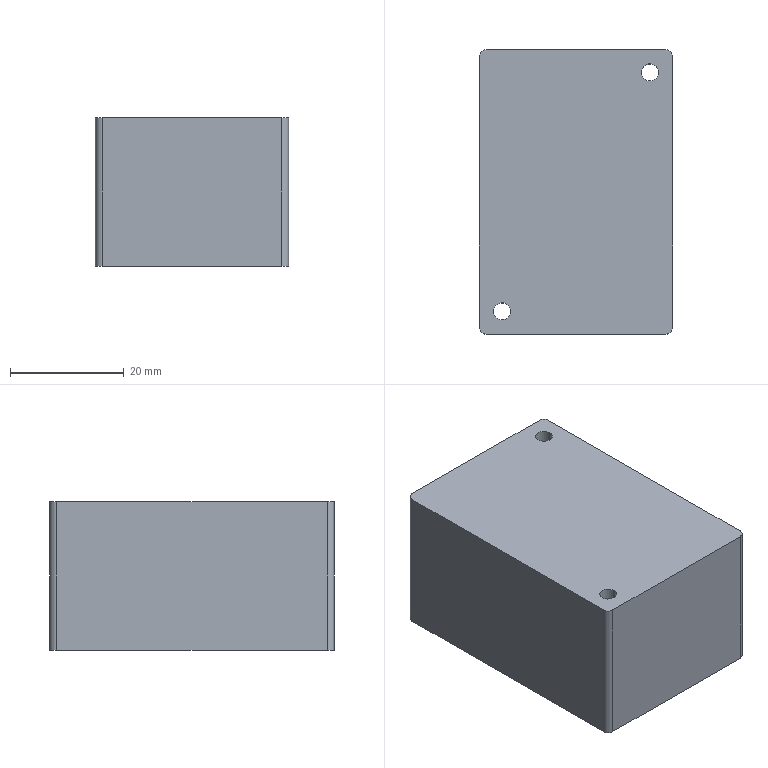Part | STEP file | 4V430C_15_Valve_Switch | 1 solid | 17 faces | box 34 x 50 x 26.2 mm | volume 44112 mm3 | cylinder 10 | plane 7 | commonest cylinder face diameters 2.4 x4 3 x4 3.4 x2
STEP:
#1=CARTESIAN_POINT('',(0.,0.,0.));
#2=DIRECTION('',(0.,0.,1.));
#3=DIRECTION('',(1.,0.,0.));
#4=AXIS2_PLACEMENT_3D('',#1,#2,#3);
#5=CARTESIAN_POINT('',(0.,22.2,-15.9));
#6=VERTEX_POINT('',#5);
#7=CARTESIAN_POINT('',(0.,25.,-15.9));
#8=VERTEX_POINT('',#7);
#9=CARTESIAN_POINT('',(0.,22.2,-15.9));
#10=DIRECTION('',(0.,1.,0.));
#11=VECTOR('',#10,1.);
#12=LINE('',#9,#11);
#13=CARTESIAN_POINT('',(0.,22.2,-17.6));
#14=DIRECTION('',(0.,1.,0.));
#15=DIRECTION('',(0.,0.,1.));
#16=AXIS2_PLACEMENT_3D('',#13,#14,#15);
#17=CYLINDRICAL_SURFACE('',#16,1.7);
#18=CARTESIAN_POINT('',(6.283,0.));
#19=DIRECTION('',(0.,1.));
#20=VECTOR('',#19,1.);
#21=LINE('',#18,#20);
#22=(GEOMETRIC_REPRESENTATION_CONTEXT(2)PARAMETRIC_REPRESENTATION_CONTEXT()REPRESENTATION_CONTEXT('',''));
#23=DEFINITIONAL_REPRESENTATION('',(#21),#22);
#24=PCURVE('',#17,#23);
#25=CARTESIAN_POINT('',(0.,22.2,-17.6));
#26=DIRECTION('',(0.,1.,0.));
#27=DIRECTION('',(0.,0.,1.));
#28=AXIS2_PLACEMENT_3D('',#25,#26,#27);
#29=CYLINDRICAL_SURFACE('',#28,1.7);
#30=CARTESIAN_POINT('',(0.,0.));
#31=DIRECTION('',(0.,1.));
#32=VECTOR('',#31,1.);
#33=LINE('',#30,#32);
#34=(GEOMETRIC_REPRESENTATION_CONTEXT(2)PARAMETRIC_REPRESENTATION_CONTEXT()REPRESENTATION_CONTEXT('',''));
#35=DEFINITIONAL_REPRESENTATION('',(#33),#34);
#36=PCURVE('',#29,#35);
#37=SURFACE_CURVE('',#12,(#24,#36),.PCURVE_S1.);
#38=EDGE_CURVE('',#6,#8,#37,.T.);
#39=ORIENTED_EDGE('',*,*,#38,.T.);
#40=CARTESIAN_POINT('',(0.,25.,-19.3));
#41=VERTEX_POINT('',#40);
#42=CARTESIAN_POINT('',(0.,25.,-17.6));
#43=DIRECTION('',(0.,1.,0.));
#44=DIRECTION('',(0.,0.,1.));
#45=AXIS2_PLACEMENT_3D('',#42,#43,#44);
#46=CIRCLE('',#45,1.7);
#47=CARTESIAN_POINT('',(0.,2.8));
#48=DIRECTION('',(1.,0.));
#49=VECTOR('',#48,1.);
#50=LINE('',#47,#49);
#51=(GEOMETRIC_REPRESENTATION_CONTEXT(2)PARAMETRIC_REPRESENTATION_CONTEXT()REPRESENTATION_CONTEXT('',''));
#52=DEFINITIONAL_REPRESENTATION('',(#50),#51);
#53=PCURVE('',#17,#52);
#54=CARTESIAN_POINT('',(15.8,25.,-26.2));
#55=DIRECTION('',(0.,1.,0.));
#56=DIRECTION('',(0.,0.,1.));
#57=AXIS2_PLACEMENT_3D('',#54,#55,#56);
#58=PLANE('',#57);
#59=CARTESIAN_POINT('',(8.6,-15.8));
#60=DIRECTION('',(1.,0.));
#61=AXIS2_PLACEMENT_2D('',#59,#60);
#62=CIRCLE('',#61,1.7);
#63=(GEOMETRIC_REPRESENTATION_CONTEXT(2)PARAMETRIC_REPRESENTATION_CONTEXT()REPRESENTATION_CONTEXT('',''));
#64=DEFINITIONAL_REPRESENTATION('',(#62),#63);
#65=PCURVE('',#58,#64);
#66=SURFACE_CURVE('',#46,(#53,#65),.PCURVE_S1.);
#67=EDGE_CURVE('',#41,#8,#66,.T.);
#68=ORIENTED_EDGE('',*,*,#67,.F.);
#69=CARTESIAN_POINT('',(0.,22.2,-19.3));
#70=VERTEX_POINT('',#69);
#71=CARTESIAN_POINT('',(0.,22.2,-19.3));
#72=DIRECTION('',(0.,1.,0.));
#73=VECTOR('',#72,1.);
#74=LINE('',#71,#73);
#75=CARTESIAN_POINT('',(3.142,0.));
#76=DIRECTION('',(0.,1.));
#77=VECTOR('',#76,1.);
#78=LINE('',#75,#77);
#79=(GEOMETRIC_REPRESENTATION_CONTEXT(2)PARAMETRIC_REPRESENTATION_CONTEXT()REPRESENTATION_CONTEXT('',''));
#80=DEFINITIONAL_REPRESENTATION('',(#78),#79);
#81=PCURVE('',#17,#80);
#82=CARTESIAN_POINT('',(3.142,0.));
#83=DIRECTION('',(0.,1.));
#84=VECTOR('',#83,1.);
#85=LINE('',#82,#84);
#86=(GEOMETRIC_REPRESENTATION_CONTEXT(2)PARAMETRIC_REPRESENTATION_CONTEXT()REPRESENTATION_CONTEXT('',''));
#87=DEFINITIONAL_REPRESENTATION('',(#85),#86);
#88=PCURVE('',#29,#87);
#89=SURFACE_CURVE('',#74,(#81,#88),.PCURVE_S1.);
#90=EDGE_CURVE('',#70,#41,#89,.T.);
#91=ORIENTED_EDGE('',*,*,#90,.F.);
#92=CARTESIAN_POINT('',(0.,22.2,-17.6));
#93=DIRECTION('',(0.,1.,0.));
#94=DIRECTION('',(0.,0.,1.));
#95=AXIS2_PLACEMENT_3D('',#92,#93,#94);
#96=CIRCLE('',#95,1.7);
#97=CARTESIAN_POINT('',(0.,0.));
#98=DIRECTION('',(1.,0.));
#99=VECTOR('',#98,1.);
#100=LINE('',#97,#99);
#101=(GEOMETRIC_REPRESENTATION_CONTEXT(2)PARAMETRIC_REPRESENTATION_CONTEXT()REPRESENTATION_CONTEXT('',''));
#102=DEFINITIONAL_REPRESENTATION('',(#100),#101);
#103=PCURVE('',#17,#102);
#104=CARTESIAN_POINT('',(0.,22.2,-19.3));
#105=DIRECTION('',(0.,1.,0.));
#106=DIRECTION('',(0.,0.,1.));
#107=AXIS2_PLACEMENT_3D('',#104,#105,#106);
#108=PLANE('',#107);
#109=CARTESIAN_POINT('',(1.7,0.));
#110=DIRECTION('',(1.,0.));
#111=AXIS2_PLACEMENT_2D('',#109,#110);
#112=CIRCLE('',#111,1.7);
#113=(GEOMETRIC_REPRESENTATION_CONTEXT(2)PARAMETRIC_REPRESENTATION_CONTEXT()REPRESENTATION_CONTEXT('',''));
#114=DEFINITIONAL_REPRESENTATION('',(#112),#113);
#115=PCURVE('',#108,#114);
#116=SURFACE_CURVE('',#96,(#103,#115),.PCURVE_S1.);
#117=EDGE_CURVE('',#70,#6,#116,.T.);
#118=ORIENTED_EDGE('',*,*,#117,.T.);
#119=EDGE_LOOP('',(#39,#68,#91,#118));
#120=FACE_BOUND('',#119,.F.);
#121=ADVANCED_FACE('',(#120),#17,.F.);
#122=CARTESIAN_POINT('',(-11.5,-21.,-26.2));
#123=VERTEX_POINT('',#122);
#124=CARTESIAN_POINT('',(-11.5,-21.,0.));
#125=VERTEX_POINT('',#124);
#126=CARTESIAN_POINT('',(-11.5,-21.,-26.2));
#127=DIRECTION('',(0.,0.,1.));
#128=VECTOR('',#127,1.);
#129=LINE('',#126,#128);
#130=CARTESIAN_POINT('',(-13.,-21.,-26.2));
#131=DIRECTION('',(0.,0.,1.));
#132=DIRECTION('',(1.,0.,0.));
#133=AXIS2_PLACEMENT_3D('',#130,#131,#132);
#134=CYLINDRICAL_SURFACE('',#133,1.5);
#135=CARTESIAN_POINT('',(6.283,0.));
#136=DIRECTION('',(0.,1.));
#137=VECTOR('',#136,1.);
#138=LINE('',#135,#137);
#139=(GEOMETRIC_REPRESENTATION_CONTEXT(2)PARAMETRIC_REPRESENTATION_CONTEXT()REPRESENTATION_CONTEXT('',''));
#140=DEFINITIONAL_REPRESENTATION('',(#138),#139);
#141=PCURVE('',#134,#140);
#142=CARTESIAN_POINT('',(-13.,-21.,-26.2));
#143=DIRECTION('',(0.,0.,1.));
#144=DIRECTION('',(1.,0.,0.));
#145=AXIS2_PLACEMENT_3D('',#142,#143,#144);
#146=CYLINDRICAL_SURFACE('',#145,1.5);
#147=CARTESIAN_POINT('',(0.,0.));
#148=DIRECTION('',(0.,1.));
#149=VECTOR('',#148,1.);
#150=LINE('',#147,#149);
#151=(GEOMETRIC_REPRESENTATION_CONTEXT(2)PARAMETRIC_REPRESENTATION_CONTEXT()REPRESENTATION_CONTEXT('',''));
#152=DEFINITIONAL_REPRESENTATION('',(#150),#151);
#153=PCURVE('',#146,#152);
#154=SURFACE_CURVE('',#129,(#141,#153),.PCURVE_S1.);
#155=EDGE_CURVE('',#123,#125,#154,.T.);
#156=ORIENTED_EDGE('',*,*,#155,.T.);
#157=CARTESIAN_POINT('',(-14.5,-21.,0.));
#158=VERTEX_POINT('',#157);
#159=CARTESIAN_POINT('',(-13.,-21.,0.));
#160=DIRECTION('',(0.,0.,1.));
#161=DIRECTION('',(1.,0.,0.));
#162=AXIS2_PLACEMENT_3D('',#159,#160,#161);
#163=CIRCLE('',#162,1.5);
#164=CARTESIAN_POINT('',(0.,26.2));
#165=DIRECTION('',(1.,0.));
#166=VECTOR('',#165,1.);
#167=LINE('',#164,#166);
#168=(GEOMETRIC_REPRESENTATION_CONTEXT(2)PARAMETRIC_REPRESENTATION_CONTEXT()REPRESENTATION_CONTEXT('',''));
#169=DEFINITIONAL_REPRESENTATION('',(#167),#168);
#170=PCURVE('',#134,#169);
#171=CARTESIAN_POINT('',(-15.8,-23.8,0.));
#172=DIRECTION('',(0.,0.,1.));
#173=DIRECTION('',(1.,0.,0.));
#174=AXIS2_PLACEMENT_3D('',#171,#172,#173);
#175=PLANE('',#174);
#176=CARTESIAN_POINT('',(2.8,2.8));
#177=DIRECTION('',(1.,0.));
#178=AXIS2_PLACEMENT_2D('',#176,#177);
#179=CIRCLE('',#178,1.5);
#180=(GEOMETRIC_REPRESENTATION_CONTEXT(2)PARAMETRIC_REPRESENTATION_CONTEXT()REPRESENTATION_CONTEXT('',''));
#181=DEFINITIONAL_REPRESENTATION('',(#179),#180);
#182=PCURVE('',#175,#181);
#183=SURFACE_CURVE('',#163,(#170,#182),.PCURVE_S1.);
#184=EDGE_CURVE('',#158,#125,#183,.T.);
#185=ORIENTED_EDGE('',*,*,#184,.F.);
#186=CARTESIAN_POINT('',(-14.5,-21.,-26.2));
#187=VERTEX_POINT('',#186);
#188=CARTESIAN_POINT('',(-14.5,-21.,-26.2));
#189=DIRECTION('',(0.,0.,1.));
#190=VECTOR('',#189,1.);
#191=LINE('',#188,#190);
#192=CARTESIAN_POINT('',(3.142,0.));
#193=DIRECTION('',(0.,1.));
#194=VECTOR('',#193,1.);
#195=LINE('',#192,#194);
#196=(GEOMETRIC_REPRESENTATION_CONTEXT(2)PARAMETRIC_REPRESENTATION_CONTEXT()REPRESENTATION_CONTEXT('',''));
#197=DEFINITIONAL_REPRESENTATION('',(#195),#196);
#198=PCURVE('',#134,#197);
#199=CARTESIAN_POINT('',(3.142,0.));
#200=DIRECTION('',(0.,1.));
#201=VECTOR('',#200,1.);
#202=LINE('',#199,#201);
#203=(GEOMETRIC_REPRESENTATION_CONTEXT(2)PARAMETRIC_REPRESENTATION_CONTEXT()REPRESENTATION_CONTEXT('',''));
#204=DEFINITIONAL_REPRESENTATION('',(#202),#203);
#205=PCURVE('',#146,#204);
#206=SURFACE_CURVE('',#191,(#198,#205),.PCURVE_S1.);
#207=EDGE_CURVE('',#187,#158,#206,.T.);
#208=ORIENTED_EDGE('',*,*,#207,.F.);
#209=CARTESIAN_POINT('',(-13.,-21.,-26.2));
#210=DIRECTION('',(0.,0.,1.));
#211=DIRECTION('',(1.,0.,0.));
#212=AXIS2_PLACEMENT_3D('',#209,#210,#211);
#213=CIRCLE('',#212,1.5);
#214=CARTESIAN_POINT('',(0.,0.));
#215=DIRECTION('',(1.,0.));
#216=VECTOR('',#215,1.);
#217=LINE('',#214,#216);
#218=(GEOMETRIC_REPRESENTATION_CONTEXT(2)PARAMETRIC_REPRESENTATION_CONTEXT()REPRESENTATION_CONTEXT('',''));
#219=DEFINITIONAL_REPRESENTATION('',(#217),#218);
#220=PCURVE('',#134,#219);
#221=CARTESIAN_POINT('',(-15.8,-23.8,-26.2));
#222=DIRECTION('',(0.,0.,1.));
#223=DIRECTION('',(1.,0.,0.));
#224=AXIS2_PLACEMENT_3D('',#221,#222,#223);
#225=PLANE('',#224);
#226=CARTESIAN_POINT('',(2.8,2.8));
#227=DIRECTION('',(1.,0.));
#228=AXIS2_PLACEMENT_2D('',#226,#227);
#229=CIRCLE('',#228,1.5);
#230=(GEOMETRIC_REPRESENTATION_CONTEXT(2)PARAMETRIC_REPRESENTATION_CONTEXT()REPRESENTATION_CONTEXT('',''));
#231=DEFINITIONAL_REPRESENTATION('',(#229),#230);
#232=PCURVE('',#225,#231);
#233=SURFACE_CURVE('',#213,(#220,#232),.PCURVE_S1.);
#234=EDGE_CURVE('',#187,#123,#233,.T.);
#235=ORIENTED_EDGE('',*,*,#234,.T.);
#236=EDGE_LOOP('',(#156,#185,#208,#235));
#237=FACE_BOUND('',#236,.F.);
#238=ADVANCED_FACE('',(#237),#134,.F.);
#239=CARTESIAN_POINT('',(14.5,21.,-26.2));
#240=VERTEX_POINT('',#239);
#241=CARTESIAN_POINT('',(14.5,21.,0.));
#242=VERTEX_POINT('',#241);
#243=CARTESIAN_POINT('',(14.5,21.,-26.2));
#244=DIRECTION('',(0.,0.,1.));
#245=VECTOR('',#244,1.);
#246=LINE('',#243,#245);
#247=CARTESIAN_POINT('',(13.,21.,-26.2));
#248=DIRECTION('',(0.,0.,1.));
#249=DIRECTION('',(1.,0.,0.));
#250=AXIS2_PLACEMENT_3D('',#247,#248,#249);
#251=CYLINDRICAL_SURFACE('',#250,1.5);
#252=CARTESIAN_POINT('',(6.283,0.));
#253=DIRECTION('',(0.,1.));
#254=VECTOR('',#253,1.);
#255=LINE('',#252,#254);
#256=(GEOMETRIC_REPRESENTATION_CONTEXT(2)PARAMETRIC_REPRESENTATION_CONTEXT()REPRESENTATION_CONTEXT('',''));
#257=DEFINITIONAL_REPRESENTATION('',(#255),#256);
#258=PCURVE('',#251,#257);
#259=CARTESIAN_POINT('',(13.,21.,-26.2));
#260=DIRECTION('',(0.,0.,1.));
#261=DIRECTION('',(1.,0.,0.));
#262=AXIS2_PLACEMENT_3D('',#259,#260,#261);
#263=CYLINDRICAL_SURFACE('',#262,1.5);
#264=CARTESIAN_POINT('',(0.,0.));
#265=DIRECTION('',(0.,1.));
#266=VECTOR('',#265,1.);
#267=LINE('',#264,#266);
#268=(GEOMETRIC_REPRESENTATION_CONTEXT(2)PARAMETRIC_REPRESENTATION_CONTEXT()REPRESENTATION_CONTEXT('',''));
#269=DEFINITIONAL_REPRESENTATION('',(#267),#268);
#270=PCURVE('',#263,#269);
#271=SURFACE_CURVE('',#246,(#258,#270),.PCURVE_S1.);
#272=EDGE_CURVE('',#240,#242,#271,.T.);
#273=ORIENTED_EDGE('',*,*,#272,.T.);
#274=CARTESIAN_POINT('',(11.5,21.,0.));
#275=VERTEX_POINT('',#274);
#276=CARTESIAN_POINT('',(13.,21.,0.));
#277=DIRECTION('',(0.,0.,1.));
#278=DIRECTION('',(1.,0.,0.));
#279=AXIS2_PLACEMENT_3D('',#276,#277,#278);
#280=CIRCLE('',#279,1.5);
#281=CARTESIAN_POINT('',(0.,26.2));
#282=DIRECTION('',(1.,0.));
#283=VECTOR('',#282,1.);
#284=LINE('',#281,#283);
#285=(GEOMETRIC_REPRESENTATION_CONTEXT(2)PARAMETRIC_REPRESENTATION_CONTEXT()REPRESENTATION_CONTEXT('',''));
#286=DEFINITIONAL_REPRESENTATION('',(#284),#285);
#287=PCURVE('',#251,#286);
#288=CARTESIAN_POINT('',(28.8,44.8));
#289=DIRECTION('',(1.,0.));
#290=AXIS2_PLACEMENT_2D('',#288,#289);
#291=CIRCLE('',#290,1.5);
#292=(GEOMETRIC_REPRESENTATION_CONTEXT(2)PARAMETRIC_REPRESENTATION_CONTEXT()REPRESENTATION_CONTEXT('',''));
#293=DEFINITIONAL_REPRESENTATION('',(#291),#292);
#294=PCURVE('',#175,#293);
#295=SURFACE_CURVE('',#280,(#287,#294),.PCURVE_S1.);
#296=EDGE_CURVE('',#275,#242,#295,.T.);
#297=ORIENTED_EDGE('',*,*,#296,.F.);
#298=CARTESIAN_POINT('',(11.5,21.,-26.2));
#299=VERTEX_POINT('',#298);
#300=CARTESIAN_POINT('',(11.5,21.,-26.2));
#301=DIRECTION('',(0.,0.,1.));
#302=VECTOR('',#301,1.);
#303=LINE('',#300,#302);
#304=CARTESIAN_POINT('',(3.142,0.));
#305=DIRECTION('',(0.,1.));
#306=VECTOR('',#305,1.);
#307=LINE('',#304,#306);
#308=(GEOMETRIC_REPRESENTATION_CONTEXT(2)PARAMETRIC_REPRESENTATION_CONTEXT()REPRESENTATION_CONTEXT('',''));
#309=DEFINITIONAL_REPRESENTATION('',(#307),#308);
#310=PCURVE('',#251,#309);
#311=CARTESIAN_POINT('',(3.142,0.));
#312=DIRECTION('',(0.,1.));
#313=VECTOR('',#312,1.);
#314=LINE('',#311,#313);
#315=(GEOMETRIC_REPRESENTATION_CONTEXT(2)PARAMETRIC_REPRESENTATION_CONTEXT()REPRESENTATION_CONTEXT('',''));
#316=DEFINITIONAL_REPRESENTATION('',(#314),#315);
#317=PCURVE('',#263,#316);
#318=SURFACE_CURVE('',#303,(#310,#317),.PCURVE_S1.);
#319=EDGE_CURVE('',#299,#275,#318,.T.);
#320=ORIENTED_EDGE('',*,*,#319,.F.);
#321=CARTESIAN_POINT('',(13.,21.,-26.2));
#322=DIRECTION('',(0.,0.,1.));
#323=DIRECTION('',(1.,0.,0.));
#324=AXIS2_PLACEMENT_3D('',#321,#322,#323);
#325=CIRCLE('',#324,1.5);
#326=CARTESIAN_POINT('',(0.,0.));
#327=DIRECTION('',(1.,0.));
#328=VECTOR('',#327,1.);
#329=LINE('',#326,#328);
#330=(GEOMETRIC_REPRESENTATION_CONTEXT(2)PARAMETRIC_REPRESENTATION_CONTEXT()REPRESENTATION_CONTEXT('',''));
#331=DEFINITIONAL_REPRESENTATION('',(#329),#330);
#332=PCURVE('',#251,#331);
#333=CARTESIAN_POINT('',(28.8,44.8));
#334=DIRECTION('',(1.,0.));
#335=AXIS2_PLACEMENT_2D('',#333,#334);
#336=CIRCLE('',#335,1.5);
#337=(GEOMETRIC_REPRESENTATION_CONTEXT(2)PARAMETRIC_REPRESENTATION_CONTEXT()REPRESENTATION_CONTEXT('',''));
#338=DEFINITIONAL_REPRESENTATION('',(#336),#337);
#339=PCURVE('',#225,#338);
#340=SURFACE_CURVE('',#325,(#332,#339),.PCURVE_S1.);
#341=EDGE_CURVE('',#299,#240,#340,.T.);
#342=ORIENTED_EDGE('',*,*,#341,.T.);
#343=EDGE_LOOP('',(#273,#297,#320,#342));
#344=FACE_BOUND('',#343,.F.);
#345=ADVANCED_FACE('',(#344),#251,.F.);
#346=CARTESIAN_POINT('',(15.8,25.,0.));
#347=VERTEX_POINT('',#346);
#348=CARTESIAN_POINT('',(-15.8,25.,0.));
#349=VERTEX_POINT('',#348);
#350=CARTESIAN_POINT('',(15.8,25.,0.));
#351=DIRECTION('',(-1.,0.,0.));
#352=VECTOR('',#351,1.);
#353=LINE('',#350,#352);
#354=CARTESIAN_POINT('',(26.2,0.));
#355=DIRECTION('',(0.,-1.));
#356=VECTOR('',#355,1.);
#357=LINE('',#354,#356);
#358=(GEOMETRIC_REPRESENTATION_CONTEXT(2)PARAMETRIC_REPRESENTATION_CONTEXT()REPRESENTATION_CONTEXT('',''));
#359=DEFINITIONAL_REPRESENTATION('',(#357),#358);
#360=PCURVE('',#58,#359);
#361=CARTESIAN_POINT('',(31.6,48.8));
#362=DIRECTION('',(-1.,0.));
#363=VECTOR('',#362,1.);
#364=LINE('',#361,#363);
#365=(GEOMETRIC_REPRESENTATION_CONTEXT(2)PARAMETRIC_REPRESENTATION_CONTEXT()REPRESENTATION_CONTEXT('',''));
#366=DEFINITIONAL_REPRESENTATION('',(#364),#365);
#367=PCURVE('',#175,#366);
#368=SURFACE_CURVE('',#353,(#360,#367),.PCURVE_S1.);
#369=EDGE_CURVE('',#347,#349,#368,.T.);
#370=ORIENTED_EDGE('',*,*,#369,.F.);
#371=CARTESIAN_POINT('',(15.8,25.,-26.2));
#372=VERTEX_POINT('',#371);
#373=CARTESIAN_POINT('',(15.8,25.,-26.2));
#374=DIRECTION('',(0.,0.,1.));
#375=VECTOR('',#374,1.);
#376=LINE('',#373,#375);
#377=CARTESIAN_POINT('',(0.,0.));
#378=DIRECTION('',(1.,0.));
#379=VECTOR('',#378,1.);
#380=LINE('',#377,#379);
#381=(GEOMETRIC_REPRESENTATION_CONTEXT(2)PARAMETRIC_REPRESENTATION_CONTEXT()REPRESENTATION_CONTEXT('',''));
#382=DEFINITIONAL_REPRESENTATION('',(#380),#381);
#383=PCURVE('',#58,#382);
#384=CARTESIAN_POINT('',(15.8,23.8,-26.2));
#385=DIRECTION('',(0.,0.,1.));
#386=DIRECTION('',(1.,0.,0.));
#387=AXIS2_PLACEMENT_3D('',#384,#385,#386);
#388=CYLINDRICAL_SURFACE('',#387,1.2);
#389=CARTESIAN_POINT('',(1.571,0.));
#390=DIRECTION('',(0.,1.));
#391=VECTOR('',#390,1.);
#392=LINE('',#389,#391);
#393=(GEOMETRIC_REPRESENTATION_CONTEXT(2)PARAMETRIC_REPRESENTATION_CONTEXT()REPRESENTATION_CONTEXT('',''));
#394=DEFINITIONAL_REPRESENTATION('',(#392),#393);
#395=PCURVE('',#388,#394);
#396=SURFACE_CURVE('',#376,(#383,#395),.PCURVE_S1.);
#397=EDGE_CURVE('',#372,#347,#396,.T.);
#398=ORIENTED_EDGE('',*,*,#397,.F.);
#399=CARTESIAN_POINT('',(-15.8,25.,-26.2));
#400=VERTEX_POINT('',#399);
#401=CARTESIAN_POINT('',(15.8,25.,-26.2));
#402=DIRECTION('',(-1.,0.,0.));
#403=VECTOR('',#402,1.);
#404=LINE('',#401,#403);
#405=CARTESIAN_POINT('',(0.,0.));
#406=DIRECTION('',(0.,-1.));
#407=VECTOR('',#406,1.);
#408=LINE('',#405,#407);
#409=(GEOMETRIC_REPRESENTATION_CONTEXT(2)PARAMETRIC_REPRESENTATION_CONTEXT()REPRESENTATION_CONTEXT('',''));
#410=DEFINITIONAL_REPRESENTATION('',(#408),#409);
#411=PCURVE('',#58,#410);
#412=CARTESIAN_POINT('',(31.6,48.8));
#413=DIRECTION('',(-1.,0.));
#414=VECTOR('',#413,1.);
#415=LINE('',#412,#414);
#416=(GEOMETRIC_REPRESENTATION_CONTEXT(2)PARAMETRIC_REPRESENTATION_CONTEXT()REPRESENTATION_CONTEXT('',''));
#417=DEFINITIONAL_REPRESENTATION('',(#415),#416);
#418=PCURVE('',#225,#417);
#419=SURFACE_CURVE('',#404,(#411,#418),.PCURVE_S1.);
#420=EDGE_CURVE('',#372,#400,#419,.T.);
#421=ORIENTED_EDGE('',*,*,#420,.T.);
#422=CARTESIAN_POINT('',(-15.8,25.,-26.2));
#423=DIRECTION('',(0.,0.,1.));
#424=VECTOR('',#423,1.);
#425=LINE('',#422,#424);
#426=CARTESIAN_POINT('',(0.,-31.6));
#427=DIRECTION('',(1.,0.));
#428=VECTOR('',#427,1.);
#429=LINE('',#426,#428);
#430=(GEOMETRIC_REPRESENTATION_CONTEXT(2)PARAMETRIC_REPRESENTATION_CONTEXT()REPRESENTATION_CONTEXT('',''));
#431=DEFINITIONAL_REPRESENTATION('',(#429),#430);
#432=PCURVE('',#58,#431);
#433=CARTESIAN_POINT('',(-15.8,23.8,-26.2));
#434=DIRECTION('',(0.,0.,1.));
#435=DIRECTION('',(1.,0.,0.));
#436=AXIS2_PLACEMENT_3D('',#433,#434,#435);
#437=CYLINDRICAL_SURFACE('',#436,1.2);
#438=CARTESIAN_POINT('',(1.571,0.));
#439=DIRECTION('',(0.,1.));
#440=VECTOR('',#439,1.);
#441=LINE('',#438,#440);
#442=(GEOMETRIC_REPRESENTATION_CONTEXT(2)PARAMETRIC_REPRESENTATION_CONTEXT()REPRESENTATION_CONTEXT('',''));
#443=DEFINITIONAL_REPRESENTATION('',(#441),#442);
#444=PCURVE('',#437,#443);
#445=SURFACE_CURVE('',#425,(#432,#444),.PCURVE_S1.);
#446=EDGE_CURVE('',#400,#349,#445,.T.);
#447=ORIENTED_EDGE('',*,*,#446,.T.);
#448=EDGE_LOOP('',(#370,#398,#421,#447));
#449=FACE_BOUND('',#448,.T.);
#450=CARTESIAN_POINT('',(0.,25.,-17.6));
#451=DIRECTION('',(0.,1.,0.));
#452=DIRECTION('',(0.,0.,1.));
#453=AXIS2_PLACEMENT_3D('',#450,#451,#452);
#454=CIRCLE('',#453,1.7);
#455=CARTESIAN_POINT('',(8.6,-15.8));
#456=DIRECTION('',(1.,0.));
#457=AXIS2_PLACEMENT_2D('',#455,#456);
#458=CIRCLE('',#457,1.7);
#459=(GEOMETRIC_REPRESENTATION_CONTEXT(2)PARAMETRIC_REPRESENTATION_CONTEXT()REPRESENTATION_CONTEXT('',''));
#460=DEFINITIONAL_REPRESENTATION('',(#458),#459);
#461=PCURVE('',#58,#460);
#462=CARTESIAN_POINT('',(0.,2.8));
#463=DIRECTION('',(1.,0.));
#464=VECTOR('',#463,1.);
#465=LINE('',#462,#464);
#466=(GEOMETRIC_REPRESENTATION_CONTEXT(2)PARAMETRIC_REPRESENTATION_CONTEXT()REPRESENTATION_CONTEXT('',''));
#467=DEFINITIONAL_REPRESENTATION('',(#465),#466);
#468=PCURVE('',#29,#467);
#469=SURFACE_CURVE('',#454,(#461,#468),.PCURVE_S1.);
#470=EDGE_CURVE('',#8,#41,#469,.T.);
#471=ORIENTED_EDGE('',*,*,#470,.F.);
#472=ORIENTED_EDGE('',*,*,#67,.F.);
#473=EDGE_LOOP('',(#471,#472));
#474=FACE_BOUND('',#473,.T.);
#475=ADVANCED_FACE('',(#449,#474),#58,.T.);
#476=CARTESIAN_POINT('',(-17.,-23.8,0.));
#477=VERTEX_POINT('',#476);
#478=CARTESIAN_POINT('',(-15.8,-25.,0.));
#479=VERTEX_POINT('',#478);
#480=CARTESIAN_POINT('',(-15.8,-23.8,0.));
#481=DIRECTION('',(0.,0.,1.));
#482=DIRECTION('',(1.,0.,0.));
#483=AXIS2_PLACEMENT_3D('',#480,#481,#482);
#484=CIRCLE('',#483,1.2);
#485=CARTESIAN_POINT('',(-15.8,-23.8,-26.2));
#486=DIRECTION('',(0.,0.,1.));
#487=DIRECTION('',(1.,0.,0.));
#488=AXIS2_PLACEMENT_3D('',#485,#486,#487);
#489=CYLINDRICAL_SURFACE('',#488,1.2);
#490=CARTESIAN_POINT('',(0.,26.2));
#491=DIRECTION('',(1.,0.));
#492=VECTOR('',#491,1.);
#493=LINE('',#490,#492);
#494=(GEOMETRIC_REPRESENTATION_CONTEXT(2)PARAMETRIC_REPRESENTATION_CONTEXT()REPRESENTATION_CONTEXT('',''));
#495=DEFINITIONAL_REPRESENTATION('',(#493),#494);
#496=PCURVE('',#489,#495);
#497=CARTESIAN_POINT('',(0.,0.));
#498=DIRECTION('',(1.,0.));
#499=AXIS2_PLACEMENT_2D('',#497,#498);
#500=CIRCLE('',#499,1.2);
#501=(GEOMETRIC_REPRESENTATION_CONTEXT(2)PARAMETRIC_REPRESENTATION_CONTEXT()REPRESENTATION_CONTEXT('',''));
#502=DEFINITIONAL_REPRESENTATION('',(#500),#501);
#503=PCURVE('',#175,#502);
#504=SURFACE_CURVE('',#484,(#496,#503),.PCURVE_S1.);
#505=EDGE_CURVE('',#477,#479,#504,.T.);
#506=ORIENTED_EDGE('',*,*,#505,.F.);
#507=CARTESIAN_POINT('',(-17.,-23.8,-26.2));
#508=VERTEX_POINT('',#507);
#509=CARTESIAN_POINT('',(-17.,-23.8,-26.2));
#510=DIRECTION('',(0.,0.,1.));
#511=VECTOR('',#510,1.);
#512=LINE('',#509,#511);
#513=CARTESIAN_POINT('',(3.142,0.));
#514=DIRECTION('',(0.,1.));
#515=VECTOR('',#514,1.);
#516=LINE('',#513,#515);
#517=(GEOMETRIC_REPRESENTATION_CONTEXT(2)PARAMETRIC_REPRESENTATION_CONTEXT()REPRESENTATION_CONTEXT('',''));
#518=DEFINITIONAL_REPRESENTATION('',(#516),#517);
#519=PCURVE('',#489,#518);
#520=CARTESIAN_POINT('',(-17.,23.8,-26.2));
#521=DIRECTION('',(-1.,0.,0.));
#522=DIRECTION('',(0.,0.,1.));
#523=AXIS2_PLACEMENT_3D('',#520,#521,#522);
#524=PLANE('',#523);
#525=CARTESIAN_POINT('',(0.,-47.6));
#526=DIRECTION('',(1.,0.));
#527=VECTOR('',#526,1.);
#528=LINE('',#525,#527);
#529=(GEOMETRIC_REPRESENTATION_CONTEXT(2)PARAMETRIC_REPRESENTATION_CONTEXT()REPRESENTATION_CONTEXT('',''));
#530=DEFINITIONAL_REPRESENTATION('',(#528),#529);
#531=PCURVE('',#524,#530);
#532=SURFACE_CURVE('',#512,(#519,#531),.PCURVE_S1.);
#533=EDGE_CURVE('',#508,#477,#532,.T.);
#534=ORIENTED_EDGE('',*,*,#533,.F.);
#535=CARTESIAN_POINT('',(-15.8,-25.,-26.2));
#536=VERTEX_POINT('',#535);
#537=CARTESIAN_POINT('',(-15.8,-23.8,-26.2));
#538=DIRECTION('',(0.,0.,1.));
#539=DIRECTION('',(1.,0.,0.));
#540=AXIS2_PLACEMENT_3D('',#537,#538,#539);
#541=CIRCLE('',#540,1.2);
#542=CARTESIAN_POINT('',(0.,0.));
#543=DIRECTION('',(1.,0.));
#544=VECTOR('',#543,1.);
#545=LINE('',#542,#544);
#546=(GEOMETRIC_REPRESENTATION_CONTEXT(2)PARAMETRIC_REPRESENTATION_CONTEXT()REPRESENTATION_CONTEXT('',''));
#547=DEFINITIONAL_REPRESENTATION('',(#545),#546);
#548=PCURVE('',#489,#547);
#549=CARTESIAN_POINT('',(0.,0.));
#550=DIRECTION('',(1.,0.));
#551=AXIS2_PLACEMENT_2D('',#549,#550);
#552=CIRCLE('',#551,1.2);
#553=(GEOMETRIC_REPRESENTATION_CONTEXT(2)PARAMETRIC_REPRESENTATION_CONTEXT()REPRESENTATION_CONTEXT('',''));
#554=DEFINITIONAL_REPRESENTATION('',(#552),#553);
#555=PCURVE('',#225,#554);
#556=SURFACE_CURVE('',#541,(#548,#555),.PCURVE_S1.);
#557=EDGE_CURVE('',#508,#536,#556,.T.);
#558=ORIENTED_EDGE('',*,*,#557,.T.);
#559=CARTESIAN_POINT('',(-15.8,-25.,-26.2));
#560=DIRECTION('',(0.,0.,1.));
#561=VECTOR('',#560,1.);
#562=LINE('',#559,#561);
#563=CARTESIAN_POINT('',(4.712,0.));
#564=DIRECTION('',(0.,1.));
#565=VECTOR('',#564,1.);
#566=LINE('',#563,#565);
#567=(GEOMETRIC_REPRESENTATION_CONTEXT(2)PARAMETRIC_REPRESENTATION_CONTEXT()REPRESENTATION_CONTEXT('',''));
#568=DEFINITIONAL_REPRESENTATION('',(#566),#567);
#569=PCURVE('',#489,#568);
#570=CARTESIAN_POINT('',(-15.8,-25.,-26.2));
#571=DIRECTION('',(0.,-1.,0.));
#572=DIRECTION('',(0.,0.,-1.));
#573=AXIS2_PLACEMENT_3D('',#570,#571,#572);
#574=PLANE('',#573);
#575=CARTESIAN_POINT('',(0.,0.));
#576=DIRECTION('',(-1.,0.));
#577=VECTOR('',#576,1.);
#578=LINE('',#575,#577);
#579=(GEOMETRIC_REPRESENTATION_CONTEXT(2)PARAMETRIC_REPRESENTATION_CONTEXT()REPRESENTATION_CONTEXT('',''));
#580=DEFINITIONAL_REPRESENTATION('',(#578),#579);
#581=PCURVE('',#574,#580);
#582=SURFACE_CURVE('',#562,(#569,#581),.PCURVE_S1.);
#583=EDGE_CURVE('',#536,#479,#582,.T.);
#584=ORIENTED_EDGE('',*,*,#583,.T.);
#585=EDGE_LOOP('',(#506,#534,#558,#584));
#586=FACE_BOUND('',#585,.T.);
#587=ADVANCED_FACE('',(#586),#489,.T.);
#588=CARTESIAN_POINT('',(-17.,23.8,0.));
#589=VERTEX_POINT('',#588);
#590=CARTESIAN_POINT('',(-17.,23.8,0.));
#591=DIRECTION('',(0.,-1.,0.));
#592=VECTOR('',#591,1.);
#593=LINE('',#590,#592);
#594=CARTESIAN_POINT('',(26.2,0.));
#595=DIRECTION('',(0.,-1.));
#596=VECTOR('',#595,1.);
#597=LINE('',#594,#596);
#598=(GEOMETRIC_REPRESENTATION_CONTEXT(2)PARAMETRIC_REPRESENTATION_CONTEXT()REPRESENTATION_CONTEXT('',''));
#599=DEFINITIONAL_REPRESENTATION('',(#597),#598);
#600=PCURVE('',#524,#599);
#601=CARTESIAN_POINT('',(-1.2,47.6));
#602=DIRECTION('',(0.,-1.));
#603=VECTOR('',#602,1.);
#604=LINE('',#601,#603);
#605=(GEOMETRIC_REPRESENTATION_CONTEXT(2)PARAMETRIC_REPRESENTATION_CONTEXT()REPRESENTATION_CONTEXT('',''));
#606=DEFINITIONAL_REPRESENTATION('',(#604),#605);
#607=PCURVE('',#175,#606);
#608=SURFACE_CURVE('',#593,(#600,#607),.PCURVE_S1.);
#609=EDGE_CURVE('',#589,#477,#608,.T.);
#610=ORIENTED_EDGE('',*,*,#609,.F.);
#611=CARTESIAN_POINT('',(-17.,23.8,-26.2));
#612=VERTEX_POINT('',#611);
#613=CARTESIAN_POINT('',(-17.,23.8,-26.2));
#614=DIRECTION('',(0.,0.,1.));
#615=VECTOR('',#614,1.);
#616=LINE('',#613,#615);
#617=CARTESIAN_POINT('',(0.,0.));
#618=DIRECTION('',(1.,0.));
#619=VECTOR('',#618,1.);
#620=LINE('',#617,#619);
#621=(GEOMETRIC_REPRESENTATION_CONTEXT(2)PARAMETRIC_REPRESENTATION_CONTEXT()REPRESENTATION_CONTEXT('',''));
#622=DEFINITIONAL_REPRESENTATION('',(#620),#621);
#623=PCURVE('',#524,#622);
#624=CARTESIAN_POINT('',(3.142,0.));
#625=DIRECTION('',(0.,1.));
#626=VECTOR('',#625,1.);
#627=LINE('',#624,#626);
#628=(GEOMETRIC_REPRESENTATION_CONTEXT(2)PARAMETRIC_REPRESENTATION_CONTEXT()REPRESENTATION_CONTEXT('',''));
#629=DEFINITIONAL_REPRESENTATION('',(#627),#628);
#630=PCURVE('',#437,#629);
#631=SURFACE_CURVE('',#616,(#623,#630),.PCURVE_S1.);
#632=EDGE_CURVE('',#612,#589,#631,.T.);
#633=ORIENTED_EDGE('',*,*,#632,.F.);
#634=CARTESIAN_POINT('',(-17.,23.8,-26.2));
#635=DIRECTION('',(0.,-1.,0.));
#636=VECTOR('',#635,1.);
#637=LINE('',#634,#636);
#638=CARTESIAN_POINT('',(0.,0.));
#639=DIRECTION('',(0.,-1.));
#640=VECTOR('',#639,1.);
#641=LINE('',#638,#640);
#642=(GEOMETRIC_REPRESENTATION_CONTEXT(2)PARAMETRIC_REPRESENTATION_CONTEXT()REPRESENTATION_CONTEXT('',''));
#643=DEFINITIONAL_REPRESENTATION('',(#641),#642);
#644=PCURVE('',#524,#643);
#645=CARTESIAN_POINT('',(-1.2,47.6));
#646=DIRECTION('',(0.,-1.));
#647=VECTOR('',#646,1.);
#648=LINE('',#645,#647);
#649=(GEOMETRIC_REPRESENTATION_CONTEXT(2)PARAMETRIC_REPRESENTATION_CONTEXT()REPRESENTATION_CONTEXT('',''));
#650=DEFINITIONAL_REPRESENTATION('',(#648),#649);
#651=PCURVE('',#225,#650);
#652=SURFACE_CURVE('',#637,(#644,#651),.PCURVE_S1.);
#653=EDGE_CURVE('',#612,#508,#652,.T.);
#654=ORIENTED_EDGE('',*,*,#653,.T.);
#655=ORIENTED_EDGE('',*,*,#533,.T.);
#656=EDGE_LOOP('',(#610,#633,#654,#655));
#657=FACE_BOUND('',#656,.T.);
#658=ADVANCED_FACE('',(#657),#524,.T.);
#659=CARTESIAN_POINT('',(-15.8,23.8,0.));
#660=DIRECTION('',(0.,0.,1.));
#661=DIRECTION('',(1.,0.,0.));
#662=AXIS2_PLACEMENT_3D('',#659,#660,#661);
#663=CIRCLE('',#662,1.2);
#664=CARTESIAN_POINT('',(0.,26.2));
#665=DIRECTION('',(1.,0.));
#666=VECTOR('',#665,1.);
#667=LINE('',#664,#666);
#668=(GEOMETRIC_REPRESENTATION_CONTEXT(2)PARAMETRIC_REPRESENTATION_CONTEXT()REPRESENTATION_CONTEXT('',''));
#669=DEFINITIONAL_REPRESENTATION('',(#667),#668);
#670=PCURVE('',#437,#669);
#671=CARTESIAN_POINT('',(0.,47.6));
#672=DIRECTION('',(1.,0.));
#673=AXIS2_PLACEMENT_2D('',#671,#672);
#674=CIRCLE('',#673,1.2);
#675=(GEOMETRIC_REPRESENTATION_CONTEXT(2)PARAMETRIC_REPRESENTATION_CONTEXT()REPRESENTATION_CONTEXT('',''));
#676=DEFINITIONAL_REPRESENTATION('',(#674),#675);
#677=PCURVE('',#175,#676);
#678=SURFACE_CURVE('',#663,(#670,#677),.PCURVE_S1.);
#679=EDGE_CURVE('',#349,#589,#678,.T.);
#680=ORIENTED_EDGE('',*,*,#679,.F.);
#681=ORIENTED_EDGE('',*,*,#446,.F.);
#682=CARTESIAN_POINT('',(-15.8,23.8,-26.2));
#683=DIRECTION('',(0.,0.,1.));
#684=DIRECTION('',(1.,0.,0.));
#685=AXIS2_PLACEMENT_3D('',#682,#683,#684);
#686=CIRCLE('',#685,1.2);
#687=CARTESIAN_POINT('',(0.,0.));
#688=DIRECTION('',(1.,0.));
#689=VECTOR('',#688,1.);
#690=LINE('',#687,#689);
#691=(GEOMETRIC_REPRESENTATION_CONTEXT(2)PARAMETRIC_REPRESENTATION_CONTEXT()REPRESENTATION_CONTEXT('',''));
#692=DEFINITIONAL_REPRESENTATION('',(#690),#691);
#693=PCURVE('',#437,#692);
#694=CARTESIAN_POINT('',(0.,47.6));
#695=DIRECTION('',(1.,0.));
#696=AXIS2_PLACEMENT_2D('',#694,#695);
#697=CIRCLE('',#696,1.2);
#698=(GEOMETRIC_REPRESENTATION_CONTEXT(2)PARAMETRIC_REPRESENTATION_CONTEXT()REPRESENTATION_CONTEXT('',''));
#699=DEFINITIONAL_REPRESENTATION('',(#697),#698);
#700=PCURVE('',#225,#699);
#701=SURFACE_CURVE('',#686,(#693,#700),.PCURVE_S1.);
#702=EDGE_CURVE('',#400,#612,#701,.T.);
#703=ORIENTED_EDGE('',*,*,#702,.T.);
#704=ORIENTED_EDGE('',*,*,#632,.T.);
#705=EDGE_LOOP('',(#680,#681,#703,#704));
#706=FACE_BOUND('',#705,.T.);
#707=ADVANCED_FACE('',(#706),#437,.T.);
#708=CARTESIAN_POINT('',(17.,23.8,0.));
#709=VERTEX_POINT('',#708);
#710=CARTESIAN_POINT('',(15.8,23.8,0.));
#711=DIRECTION('',(0.,0.,1.));
#712=DIRECTION('',(1.,0.,0.));
#713=AXIS2_PLACEMENT_3D('',#710,#711,#712);
#714=CIRCLE('',#713,1.2);
#715=CARTESIAN_POINT('',(0.,26.2));
#716=DIRECTION('',(1.,0.));
#717=VECTOR('',#716,1.);
#718=LINE('',#715,#717);
#719=(GEOMETRIC_REPRESENTATION_CONTEXT(2)PARAMETRIC_REPRESENTATION_CONTEXT()REPRESENTATION_CONTEXT('',''));
#720=DEFINITIONAL_REPRESENTATION('',(#718),#719);
#721=PCURVE('',#388,#720);
#722=CARTESIAN_POINT('',(31.6,47.6));
#723=DIRECTION('',(1.,0.));
#724=AXIS2_PLACEMENT_2D('',#722,#723);
#725=CIRCLE('',#724,1.2);
#726=(GEOMETRIC_REPRESENTATION_CONTEXT(2)PARAMETRIC_REPRESENTATION_CONTEXT()REPRESENTATION_CONTEXT('',''));
#727=DEFINITIONAL_REPRESENTATION('',(#725),#726);
#728=PCURVE('',#175,#727);
#729=SURFACE_CURVE('',#714,(#721,#728),.PCURVE_S1.);
#730=EDGE_CURVE('',#709,#347,#729,.T.);
#731=ORIENTED_EDGE('',*,*,#730,.F.);
#732=CARTESIAN_POINT('',(17.,23.8,-26.2));
#733=VERTEX_POINT('',#732);
#734=CARTESIAN_POINT('',(17.,23.8,-26.2));
#735=DIRECTION('',(0.,0.,1.));
#736=VECTOR('',#735,1.);
#737=LINE('',#734,#736);
#738=CARTESIAN_POINT('',(0.,0.));
#739=DIRECTION('',(0.,1.));
#740=VECTOR('',#739,1.);
#741=LINE('',#738,#740);
#742=(GEOMETRIC_REPRESENTATION_CONTEXT(2)PARAMETRIC_REPRESENTATION_CONTEXT()REPRESENTATION_CONTEXT('',''));
#743=DEFINITIONAL_REPRESENTATION('',(#741),#742);
#744=PCURVE('',#388,#743);
#745=CARTESIAN_POINT('',(17.,-23.8,-26.2));
#746=DIRECTION('',(1.,0.,0.));
#747=DIRECTION('',(0.,0.,-1.));
#748=AXIS2_PLACEMENT_3D('',#745,#746,#747);
#749=PLANE('',#748);
#750=CARTESIAN_POINT('',(0.,47.6));
#751=DIRECTION('',(-1.,0.));
#752=VECTOR('',#751,1.);
#753=LINE('',#750,#752);
#754=(GEOMETRIC_REPRESENTATION_CONTEXT(2)PARAMETRIC_REPRESENTATION_CONTEXT()REPRESENTATION_CONTEXT('',''));
#755=DEFINITIONAL_REPRESENTATION('',(#753),#754);
#756=PCURVE('',#749,#755);
#757=SURFACE_CURVE('',#737,(#744,#756),.PCURVE_S1.);
#758=EDGE_CURVE('',#733,#709,#757,.T.);
#759=ORIENTED_EDGE('',*,*,#758,.F.);
#760=CARTESIAN_POINT('',(15.8,23.8,-26.2));
#761=DIRECTION('',(0.,0.,1.));
#762=DIRECTION('',(1.,0.,0.));
#763=AXIS2_PLACEMENT_3D('',#760,#761,#762);
#764=CIRCLE('',#763,1.2);
#765=CARTESIAN_POINT('',(0.,0.));
#766=DIRECTION('',(1.,0.));
#767=VECTOR('',#766,1.);
#768=LINE('',#765,#767);
#769=(GEOMETRIC_REPRESENTATION_CONTEXT(2)PARAMETRIC_REPRESENTATION_CONTEXT()REPRESENTATION_CONTEXT('',''));
#770=DEFINITIONAL_REPRESENTATION('',(#768),#769);
#771=PCURVE('',#388,#770);
#772=CARTESIAN_POINT('',(31.6,47.6));
#773=DIRECTION('',(1.,0.));
#774=AXIS2_PLACEMENT_2D('',#772,#773);
#775=CIRCLE('',#774,1.2);
#776=(GEOMETRIC_REPRESENTATION_CONTEXT(2)PARAMETRIC_REPRESENTATION_CONTEXT()REPRESENTATION_CONTEXT('',''));
#777=DEFINITIONAL_REPRESENTATION('',(#775),#776);
#778=PCURVE('',#225,#777);
#779=SURFACE_CURVE('',#764,(#771,#778),.PCURVE_S1.);
#780=EDGE_CURVE('',#733,#372,#779,.T.);
#781=ORIENTED_EDGE('',*,*,#780,.T.);
#782=ORIENTED_EDGE('',*,*,#397,.T.);
#783=EDGE_LOOP('',(#731,#759,#781,#782));
#784=FACE_BOUND('',#783,.T.);
#785=ADVANCED_FACE('',(#784),#388,.T.);
#786=CARTESIAN_POINT('',(17.,-23.8,0.));
#787=VERTEX_POINT('',#786);
#788=CARTESIAN_POINT('',(17.,-23.8,0.));
#789=DIRECTION('',(0.,1.,0.));
#790=VECTOR('',#789,1.);
#791=LINE('',#788,#790);
#792=CARTESIAN_POINT('',(-26.2,0.));
#793=DIRECTION('',(0.,1.));
#794=VECTOR('',#793,1.);
#795=LINE('',#792,#794);
#796=(GEOMETRIC_REPRESENTATION_CONTEXT(2)PARAMETRIC_REPRESENTATION_CONTEXT()REPRESENTATION_CONTEXT('',''));
#797=DEFINITIONAL_REPRESENTATION('',(#795),#796);
#798=PCURVE('',#749,#797);
#799=CARTESIAN_POINT('',(32.8,0.));
#800=DIRECTION('',(0.,1.));
#801=VECTOR('',#800,1.);
#802=LINE('',#799,#801);
#803=(GEOMETRIC_REPRESENTATION_CONTEXT(2)PARAMETRIC_REPRESENTATION_CONTEXT()REPRESENTATION_CONTEXT('',''));
#804=DEFINITIONAL_REPRESENTATION('',(#802),#803);
#805=PCURVE('',#175,#804);
#806=SURFACE_CURVE('',#791,(#798,#805),.PCURVE_S1.);
#807=EDGE_CURVE('',#787,#709,#806,.T.);
#808=ORIENTED_EDGE('',*,*,#807,.F.);
#809=CARTESIAN_POINT('',(17.,-23.8,-26.2));
#810=VERTEX_POINT('',#809);
#811=CARTESIAN_POINT('',(17.,-23.8,-26.2));
#812=DIRECTION('',(0.,0.,1.));
#813=VECTOR('',#812,1.);
#814=LINE('',#811,#813);
#815=CARTESIAN_POINT('',(0.,0.));
#816=DIRECTION('',(-1.,0.));
#817=VECTOR('',#816,1.);
#818=LINE('',#815,#817);
#819=(GEOMETRIC_REPRESENTATION_CONTEXT(2)PARAMETRIC_REPRESENTATION_CONTEXT()REPRESENTATION_CONTEXT('',''));
#820=DEFINITIONAL_REPRESENTATION('',(#818),#819);
#821=PCURVE('',#749,#820);
#822=CARTESIAN_POINT('',(15.8,-23.8,-26.2));
#823=DIRECTION('',(0.,0.,1.));
#824=DIRECTION('',(1.,0.,0.));
#825=AXIS2_PLACEMENT_3D('',#822,#823,#824);
#826=CYLINDRICAL_SURFACE('',#825,1.2);
#827=CARTESIAN_POINT('',(6.283,0.));
#828=DIRECTION('',(0.,1.));
#829=VECTOR('',#828,1.);
#830=LINE('',#827,#829);
#831=(GEOMETRIC_REPRESENTATION_CONTEXT(2)PARAMETRIC_REPRESENTATION_CONTEXT()REPRESENTATION_CONTEXT('',''));
#832=DEFINITIONAL_REPRESENTATION('',(#830),#831);
#833=PCURVE('',#826,#832);
#834=SURFACE_CURVE('',#814,(#821,#833),.PCURVE_S1.);
#835=EDGE_CURVE('',#810,#787,#834,.T.);
#836=ORIENTED_EDGE('',*,*,#835,.F.);
#837=CARTESIAN_POINT('',(17.,-23.8,-26.2));
#838=DIRECTION('',(0.,1.,0.));
#839=VECTOR('',#838,1.);
#840=LINE('',#837,#839);
#841=CARTESIAN_POINT('',(0.,0.));
#842=DIRECTION('',(0.,1.));
#843=VECTOR('',#842,1.);
#844=LINE('',#841,#843);
#845=(GEOMETRIC_REPRESENTATION_CONTEXT(2)PARAMETRIC_REPRESENTATION_CONTEXT()REPRESENTATION_CONTEXT('',''));
#846=DEFINITIONAL_REPRESENTATION('',(#844),#845);
#847=PCURVE('',#749,#846);
#848=CARTESIAN_POINT('',(32.8,0.));
#849=DIRECTION('',(0.,1.));
#850=VECTOR('',#849,1.);
#851=LINE('',#848,#850);
#852=(GEOMETRIC_REPRESENTATION_CONTEXT(2)PARAMETRIC_REPRESENTATION_CONTEXT()REPRESENTATION_CONTEXT('',''));
#853=DEFINITIONAL_REPRESENTATION('',(#851),#852);
#854=PCURVE('',#225,#853);
#855=SURFACE_CURVE('',#840,(#847,#854),.PCURVE_S1.);
#856=EDGE_CURVE('',#810,#733,#855,.T.);
#857=ORIENTED_EDGE('',*,*,#856,.T.);
#858=ORIENTED_EDGE('',*,*,#758,.T.);
#859=EDGE_LOOP('',(#808,#836,#857,#858));
#860=FACE_BOUND('',#859,.T.);
#861=ADVANCED_FACE('',(#860),#749,.T.);
#862=CARTESIAN_POINT('',(15.8,-25.,0.));
#863=VERTEX_POINT('',#862);
#864=CARTESIAN_POINT('',(15.8,-23.8,0.));
#865=DIRECTION('',(0.,0.,1.));
#866=DIRECTION('',(1.,0.,0.));
#867=AXIS2_PLACEMENT_3D('',#864,#865,#866);
#868=CIRCLE('',#867,1.2);
#869=CARTESIAN_POINT('',(0.,26.2));
#870=DIRECTION('',(1.,0.));
#871=VECTOR('',#870,1.);
#872=LINE('',#869,#871);
#873=(GEOMETRIC_REPRESENTATION_CONTEXT(2)PARAMETRIC_REPRESENTATION_CONTEXT()REPRESENTATION_CONTEXT('',''));
#874=DEFINITIONAL_REPRESENTATION('',(#872),#873);
#875=PCURVE('',#826,#874);
#876=CARTESIAN_POINT('',(31.6,0.));
#877=DIRECTION('',(1.,0.));
#878=AXIS2_PLACEMENT_2D('',#876,#877);
#879=CIRCLE('',#878,1.2);
#880=(GEOMETRIC_REPRESENTATION_CONTEXT(2)PARAMETRIC_REPRESENTATION_CONTEXT()REPRESENTATION_CONTEXT('',''));
#881=DEFINITIONAL_REPRESENTATION('',(#879),#880);
#882=PCURVE('',#175,#881);
#883=SURFACE_CURVE('',#868,(#875,#882),.PCURVE_S1.);
#884=EDGE_CURVE('',#863,#787,#883,.T.);
#885=ORIENTED_EDGE('',*,*,#884,.F.);
#886=CARTESIAN_POINT('',(15.8,-25.,-26.2));
#887=VERTEX_POINT('',#886);
#888=CARTESIAN_POINT('',(15.8,-25.,-26.2));
#889=DIRECTION('',(0.,0.,1.));
#890=VECTOR('',#889,1.);
#891=LINE('',#888,#890);
#892=CARTESIAN_POINT('',(4.712,0.));
#893=DIRECTION('',(0.,1.));
#894=VECTOR('',#893,1.);
#895=LINE('',#892,#894);
#896=(GEOMETRIC_REPRESENTATION_CONTEXT(2)PARAMETRIC_REPRESENTATION_CONTEXT()REPRESENTATION_CONTEXT('',''));
#897=DEFINITIONAL_REPRESENTATION('',(#895),#896);
#898=PCURVE('',#826,#897);
#899=CARTESIAN_POINT('',(0.,31.6));
#900=DIRECTION('',(-1.,0.));
#901=VECTOR('',#900,1.);
#902=LINE('',#899,#901);
#903=(GEOMETRIC_REPRESENTATION_CONTEXT(2)PARAMETRIC_REPRESENTATION_CONTEXT()REPRESENTATION_CONTEXT('',''));
#904=DEFINITIONAL_REPRESENTATION('',(#902),#903);
#905=PCURVE('',#574,#904);
#906=SURFACE_CURVE('',#891,(#898,#905),.PCURVE_S1.);
#907=EDGE_CURVE('',#887,#863,#906,.T.);
#908=ORIENTED_EDGE('',*,*,#907,.F.);
#909=CARTESIAN_POINT('',(15.8,-23.8,-26.2));
#910=DIRECTION('',(0.,0.,1.));
#911=DIRECTION('',(1.,0.,0.));
#912=AXIS2_PLACEMENT_3D('',#909,#910,#911);
#913=CIRCLE('',#912,1.2);
#914=CARTESIAN_POINT('',(0.,0.));
#915=DIRECTION('',(1.,0.));
#916=VECTOR('',#915,1.);
#917=LINE('',#914,#916);
#918=(GEOMETRIC_REPRESENTATION_CONTEXT(2)PARAMETRIC_REPRESENTATION_CONTEXT()REPRESENTATION_CONTEXT('',''));
#919=DEFINITIONAL_REPRESENTATION('',(#917),#918);
#920=PCURVE('',#826,#919);
#921=CARTESIAN_POINT('',(31.6,0.));
#922=DIRECTION('',(1.,0.));
#923=AXIS2_PLACEMENT_2D('',#921,#922);
#924=CIRCLE('',#923,1.2);
#925=(GEOMETRIC_REPRESENTATION_CONTEXT(2)PARAMETRIC_REPRESENTATION_CONTEXT()REPRESENTATION_CONTEXT('',''));
#926=DEFINITIONAL_REPRESENTATION('',(#924),#925);
#927=PCURVE('',#225,#926);
#928=SURFACE_CURVE('',#913,(#920,#927),.PCURVE_S1.);
#929=EDGE_CURVE('',#887,#810,#928,.T.);
#930=ORIENTED_EDGE('',*,*,#929,.T.);
#931=ORIENTED_EDGE('',*,*,#835,.T.);
#932=EDGE_LOOP('',(#885,#908,#930,#931));
#933=FACE_BOUND('',#932,.T.);
#934=ADVANCED_FACE('',(#933),#826,.T.);
#935=CARTESIAN_POINT('',(-15.8,-25.,0.));
#936=DIRECTION('',(1.,0.,0.));
#937=VECTOR('',#936,1.);
#938=LINE('',#935,#937);
#939=CARTESIAN_POINT('',(-26.2,0.));
#940=DIRECTION('',(0.,1.));
#941=VECTOR('',#940,1.);
#942=LINE('',#939,#941);
#943=(GEOMETRIC_REPRESENTATION_CONTEXT(2)PARAMETRIC_REPRESENTATION_CONTEXT()REPRESENTATION_CONTEXT('',''));
#944=DEFINITIONAL_REPRESENTATION('',(#942),#943);
#945=PCURVE('',#574,#944);
#946=CARTESIAN_POINT('',(0.,-1.2));
#947=DIRECTION('',(1.,0.));
#948=VECTOR('',#947,1.);
#949=LINE('',#946,#948);
#950=(GEOMETRIC_REPRESENTATION_CONTEXT(2)PARAMETRIC_REPRESENTATION_CONTEXT()REPRESENTATION_CONTEXT('',''));
#951=DEFINITIONAL_REPRESENTATION('',(#949),#950);
#952=PCURVE('',#175,#951);
#953=SURFACE_CURVE('',#938,(#945,#952),.PCURVE_S1.);
#954=EDGE_CURVE('',#479,#863,#953,.T.);
#955=ORIENTED_EDGE('',*,*,#954,.F.);
#956=ORIENTED_EDGE('',*,*,#583,.F.);
#957=CARTESIAN_POINT('',(-15.8,-25.,-26.2));
#958=DIRECTION('',(1.,0.,0.));
#959=VECTOR('',#958,1.);
#960=LINE('',#957,#959);
#961=CARTESIAN_POINT('',(0.,0.));
#962=DIRECTION('',(0.,1.));
#963=VECTOR('',#962,1.);
#964=LINE('',#961,#963);
#965=(GEOMETRIC_REPRESENTATION_CONTEXT(2)PARAMETRIC_REPRESENTATION_CONTEXT()REPRESENTATION_CONTEXT('',''));
#966=DEFINITIONAL_REPRESENTATION('',(#964),#965);
#967=PCURVE('',#574,#966);
#968=CARTESIAN_POINT('',(0.,-1.2));
#969=DIRECTION('',(1.,0.));
#970=VECTOR('',#969,1.);
#971=LINE('',#968,#970);
#972=(GEOMETRIC_REPRESENTATION_CONTEXT(2)PARAMETRIC_REPRESENTATION_CONTEXT()REPRESENTATION_CONTEXT('',''));
#973=DEFINITIONAL_REPRESENTATION('',(#971),#972);
#974=PCURVE('',#225,#973);
#975=SURFACE_CURVE('',#960,(#967,#974),.PCURVE_S1.);
#976=EDGE_CURVE('',#536,#887,#975,.T.);
#977=ORIENTED_EDGE('',*,*,#976,.T.);
#978=ORIENTED_EDGE('',*,*,#907,.T.);
#979=EDGE_LOOP('',(#955,#956,#977,#978));
#980=FACE_BOUND('',#979,.T.);
#981=ADVANCED_FACE('',(#980),#574,.T.);
#982=CARTESIAN_POINT('',(-13.,-21.,-26.2));
#983=DIRECTION('',(0.,0.,1.));
#984=DIRECTION('',(1.,0.,0.));
#985=AXIS2_PLACEMENT_3D('',#982,#983,#984);
#986=CIRCLE('',#985,1.5);
#987=CARTESIAN_POINT('',(2.8,2.8));
#988=DIRECTION('',(1.,0.));
#989=AXIS2_PLACEMENT_2D('',#987,#988);
#990=CIRCLE('',#989,1.5);
#991=(GEOMETRIC_REPRESENTATION_CONTEXT(2)PARAMETRIC_REPRESENTATION_CONTEXT()REPRESENTATION_CONTEXT('',''));
#992=DEFINITIONAL_REPRESENTATION('',(#990),#991);
#993=PCURVE('',#225,#992);
#994=CARTESIAN_POINT('',(0.,0.));
#995=DIRECTION('',(1.,0.));
#996=VECTOR('',#995,1.);
#997=LINE('',#994,#996);
#998=(GEOMETRIC_REPRESENTATION_CONTEXT(2)PARAMETRIC_REPRESENTATION_CONTEXT()REPRESENTATION_CONTEXT('',''));
#999=DEFINITIONAL_REPRESENTATION('',(#997),#998);
#1000=PCURVE('',#146,#999);
#1001=SURFACE_CURVE('',#986,(#993,#1000),.PCURVE_S1.);
#1002=EDGE_CURVE('',#123,#187,#1001,.T.);
#1003=ORIENTED_EDGE('',*,*,#1002,.T.);
#1004=ORIENTED_EDGE('',*,*,#234,.T.);
#1005=EDGE_LOOP('',(#1003,#1004));
#1006=FACE_BOUND('',#1005,.T.);
#1007=CARTESIAN_POINT('',(13.,21.,-26.2));
#1008=DIRECTION('',(0.,0.,1.));
#1009=DIRECTION('',(1.,0.,0.));
#1010=AXIS2_PLACEMENT_3D('',#1007,#1008,#1009);
#1011=CIRCLE('',#1010,1.5);
#1012=CARTESIAN_POINT('',(28.8,44.8));
#1013=DIRECTION('',(1.,0.));
#1014=AXIS2_PLACEMENT_2D('',#1012,#1013);
#1015=CIRCLE('',#1014,1.5);
#1016=(GEOMETRIC_REPRESENTATION_CONTEXT(2)PARAMETRIC_REPRESENTATION_CONTEXT()REPRESENTATION_CONTEXT('',''));
#1017=DEFINITIONAL_REPRESENTATION('',(#1015),#1016);
#1018=PCURVE('',#225,#1017);
#1019=CARTESIAN_POINT('',(0.,0.));
#1020=DIRECTION('',(1.,0.));
#1021=VECTOR('',#1020,1.);
#1022=LINE('',#1019,#1021);
#1023=(GEOMETRIC_REPRESENTATION_CONTEXT(2)PARAMETRIC_REPRESENTATION_CONTEXT()REPRESENTATION_CONTEXT('',''));
#1024=DEFINITIONAL_REPRESENTATION('',(#1022),#1023);
#1025=PCURVE('',#263,#1024);
#1026=SURFACE_CURVE('',#1011,(#1018,#1025),.PCURVE_S1.);
#1027=EDGE_CURVE('',#240,#299,#1026,.T.);
#1028=ORIENTED_EDGE('',*,*,#1027,.T.);
#1029=ORIENTED_EDGE('',*,*,#341,.T.);
#1030=EDGE_LOOP('',(#1028,#1029));
#1031=FACE_BOUND('',#1030,.T.);
#1032=ORIENTED_EDGE('',*,*,#557,.F.);
#1033=ORIENTED_EDGE('',*,*,#653,.F.);
#1034=ORIENTED_EDGE('',*,*,#702,.F.);
#1035=ORIENTED_EDGE('',*,*,#420,.F.);
#1036=ORIENTED_EDGE('',*,*,#780,.F.);
#1037=ORIENTED_EDGE('',*,*,#856,.F.);
#1038=ORIENTED_EDGE('',*,*,#929,.F.);
#1039=ORIENTED_EDGE('',*,*,#976,.F.);
#1040=EDGE_LOOP('',(#1032,#1033,#1034,#1035,#1036,#1037,#1038,#1039));
#1041=FACE_BOUND('',#1040,.T.);
#1042=ADVANCED_FACE('',(#1006,#1031,#1041),#225,.F.);
#1043=CARTESIAN_POINT('',(-13.,-21.,0.));
#1044=DIRECTION('',(0.,0.,1.));
#1045=DIRECTION('',(1.,0.,0.));
#1046=AXIS2_PLACEMENT_3D('',#1043,#1044,#1045);
#1047=CIRCLE('',#1046,1.5);
#1048=CARTESIAN_POINT('',(2.8,2.8));
#1049=DIRECTION('',(1.,0.));
#1050=AXIS2_PLACEMENT_2D('',#1048,#1049);
#1051=CIRCLE('',#1050,1.5);
#1052=(GEOMETRIC_REPRESENTATION_CONTEXT(2)PARAMETRIC_REPRESENTATION_CONTEXT()REPRESENTATION_CONTEXT('',''));
#1053=DEFINITIONAL_REPRESENTATION('',(#1051),#1052);
#1054=PCURVE('',#175,#1053);
#1055=CARTESIAN_POINT('',(0.,26.2));
#1056=DIRECTION('',(1.,0.));
#1057=VECTOR('',#1056,1.);
#1058=LINE('',#1055,#1057);
#1059=(GEOMETRIC_REPRESENTATION_CONTEXT(2)PARAMETRIC_REPRESENTATION_CONTEXT()REPRESENTATION_CONTEXT('',''));
#1060=DEFINITIONAL_REPRESENTATION('',(#1058),#1059);
#1061=PCURVE('',#146,#1060);
#1062=SURFACE_CURVE('',#1047,(#1054,#1061),.PCURVE_S1.);
#1063=EDGE_CURVE('',#125,#158,#1062,.T.);
#1064=ORIENTED_EDGE('',*,*,#1063,.F.);
#1065=ORIENTED_EDGE('',*,*,#184,.F.);
#1066=EDGE_LOOP('',(#1064,#1065));
#1067=FACE_BOUND('',#1066,.T.);
#1068=CARTESIAN_POINT('',(13.,21.,0.));
#1069=DIRECTION('',(0.,0.,1.));
#1070=DIRECTION('',(1.,0.,0.));
#1071=AXIS2_PLACEMENT_3D('',#1068,#1069,#1070);
#1072=CIRCLE('',#1071,1.5);
#1073=CARTESIAN_POINT('',(28.8,44.8));
#1074=DIRECTION('',(1.,0.));
#1075=AXIS2_PLACEMENT_2D('',#1073,#1074);
#1076=CIRCLE('',#1075,1.5);
#1077=(GEOMETRIC_REPRESENTATION_CONTEXT(2)PARAMETRIC_REPRESENTATION_CONTEXT()REPRESENTATION_CONTEXT('',''));
#1078=DEFINITIONAL_REPRESENTATION('',(#1076),#1077);
#1079=PCURVE('',#175,#1078);
#1080=CARTESIAN_POINT('',(0.,26.2));
#1081=DIRECTION('',(1.,0.));
#1082=VECTOR('',#1081,1.);
#1083=LINE('',#1080,#1082);
#1084=(GEOMETRIC_REPRESENTATION_CONTEXT(2)PARAMETRIC_REPRESENTATION_CONTEXT()REPRESENTATION_CONTEXT('',''));
#1085=DEFINITIONAL_REPRESENTATION('',(#1083),#1084);
#1086=PCURVE('',#263,#1085);
#1087=SURFACE_CURVE('',#1072,(#1079,#1086),.PCURVE_S1.);
#1088=EDGE_CURVE('',#242,#275,#1087,.T.);
#1089=ORIENTED_EDGE('',*,*,#1088,.F.);
#1090=ORIENTED_EDGE('',*,*,#296,.F.);
#1091=EDGE_LOOP('',(#1089,#1090));
#1092=FACE_BOUND('',#1091,.T.);
#1093=ORIENTED_EDGE('',*,*,#505,.T.);
#1094=ORIENTED_EDGE('',*,*,#954,.T.);
#1095=ORIENTED_EDGE('',*,*,#884,.T.);
#1096=ORIENTED_EDGE('',*,*,#807,.T.);
#1097=ORIENTED_EDGE('',*,*,#730,.T.);
#1098=ORIENTED_EDGE('',*,*,#369,.T.);
#1099=ORIENTED_EDGE('',*,*,#679,.T.);
#1100=ORIENTED_EDGE('',*,*,#609,.T.);
#1101=EDGE_LOOP('',(#1093,#1094,#1095,#1096,#1097,#1098,#1099,#1100));
#1102=FACE_BOUND('',#1101,.T.);
#1103=ADVANCED_FACE('',(#1067,#1092,#1102),#175,.T.);
#1104=ORIENTED_EDGE('',*,*,#1088,.F.);
#1105=ORIENTED_EDGE('',*,*,#272,.F.);
#1106=ORIENTED_EDGE('',*,*,#1027,.T.);
#1107=ORIENTED_EDGE('',*,*,#319,.T.);
#1108=EDGE_LOOP('',(#1104,#1105,#1106,#1107));
#1109=FACE_BOUND('',#1108,.F.);
#1110=ADVANCED_FACE('',(#1109),#263,.F.);
#1111=ORIENTED_EDGE('',*,*,#1063,.F.);
#1112=ORIENTED_EDGE('',*,*,#155,.F.);
#1113=ORIENTED_EDGE('',*,*,#1002,.T.);
#1114=ORIENTED_EDGE('',*,*,#207,.T.);
#1115=EDGE_LOOP('',(#1111,#1112,#1113,#1114));
#1116=FACE_BOUND('',#1115,.F.);
#1117=ADVANCED_FACE('',(#1116),#146,.F.);
#1118=ORIENTED_EDGE('',*,*,#470,.F.);
#1119=ORIENTED_EDGE('',*,*,#38,.F.);
#1120=CARTESIAN_POINT('',(0.,22.2,-17.6));
#1121=DIRECTION('',(0.,1.,0.));
#1122=DIRECTION('',(0.,0.,1.));
#1123=AXIS2_PLACEMENT_3D('',#1120,#1121,#1122);
#1124=CIRCLE('',#1123,1.7);
#1125=CARTESIAN_POINT('',(0.,0.));
#1126=DIRECTION('',(1.,0.));
#1127=VECTOR('',#1126,1.);
#1128=LINE('',#1125,#1127);
#1129=(GEOMETRIC_REPRESENTATION_CONTEXT(2)PARAMETRIC_REPRESENTATION_CONTEXT()REPRESENTATION_CONTEXT('',''));
#1130=DEFINITIONAL_REPRESENTATION('',(#1128),#1129);
#1131=PCURVE('',#29,#1130);
#1132=CARTESIAN_POINT('',(1.7,0.));
#1133=DIRECTION('',(1.,0.));
#1134=AXIS2_PLACEMENT_2D('',#1132,#1133);
#1135=CIRCLE('',#1134,1.7);
#1136=(GEOMETRIC_REPRESENTATION_CONTEXT(2)PARAMETRIC_REPRESENTATION_CONTEXT()REPRESENTATION_CONTEXT('',''));
#1137=DEFINITIONAL_REPRESENTATION('',(#1135),#1136);
#1138=PCURVE('',#108,#1137);
#1139=SURFACE_CURVE('',#1124,(#1131,#1138),.PCURVE_S1.);
#1140=EDGE_CURVE('',#6,#70,#1139,.T.);
#1141=ORIENTED_EDGE('',*,*,#1140,.T.);
#1142=ORIENTED_EDGE('',*,*,#90,.T.);
#1143=EDGE_LOOP('',(#1118,#1119,#1141,#1142));
#1144=FACE_BOUND('',#1143,.F.);
#1145=ADVANCED_FACE('',(#1144),#29,.F.);
#1146=ORIENTED_EDGE('',*,*,#1140,.T.);
#1147=ORIENTED_EDGE('',*,*,#117,.T.);
#1148=EDGE_LOOP('',(#1146,#1147));
#1149=FACE_BOUND('',#1148,.T.);
#1150=ADVANCED_FACE('',(#1149),#108,.T.);
#1151=CLOSED_SHELL('',(#121,#238,#345,#475,#587,#658,#707,#785,#861,#934,#981,#1042,#1103,#1110,#1117,#1145,#1150));
#1152=MANIFOLD_SOLID_BREP('',#1151);
#1153=(LENGTH_UNIT()NAMED_UNIT(*)SI_UNIT(.MILLI.,.METRE.));
#1154=UNCERTAINTY_MEASURE_WITH_UNIT(LENGTH_MEASURE(0.0000001),#1153,'','');
#1155=(NAMED_UNIT(*)PLANE_ANGLE_UNIT()SI_UNIT($,.RADIAN.));
#1156=(NAMED_UNIT(*)SI_UNIT($,.STERADIAN.)SOLID_ANGLE_UNIT());
#1157=(GEOMETRIC_REPRESENTATION_CONTEXT(3)GLOBAL_UNCERTAINTY_ASSIGNED_CONTEXT((#1154))GLOBAL_UNIT_ASSIGNED_CONTEXT((#1153,#1155,#1156))REPRESENTATION_CONTEXT('',''));
#1158=ADVANCED_BREP_SHAPE_REPRESENTATION('',(#4,#1152),#1157);